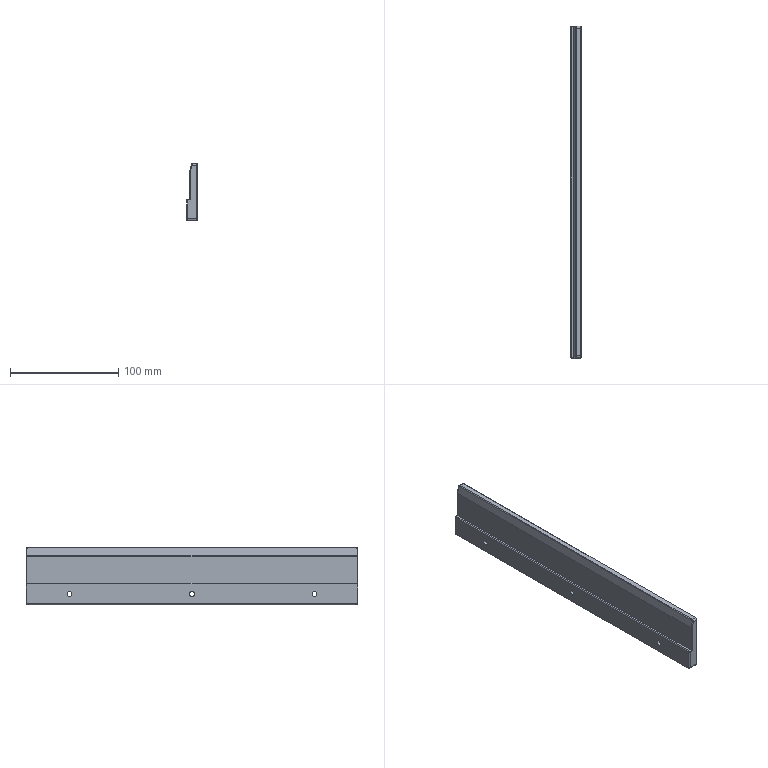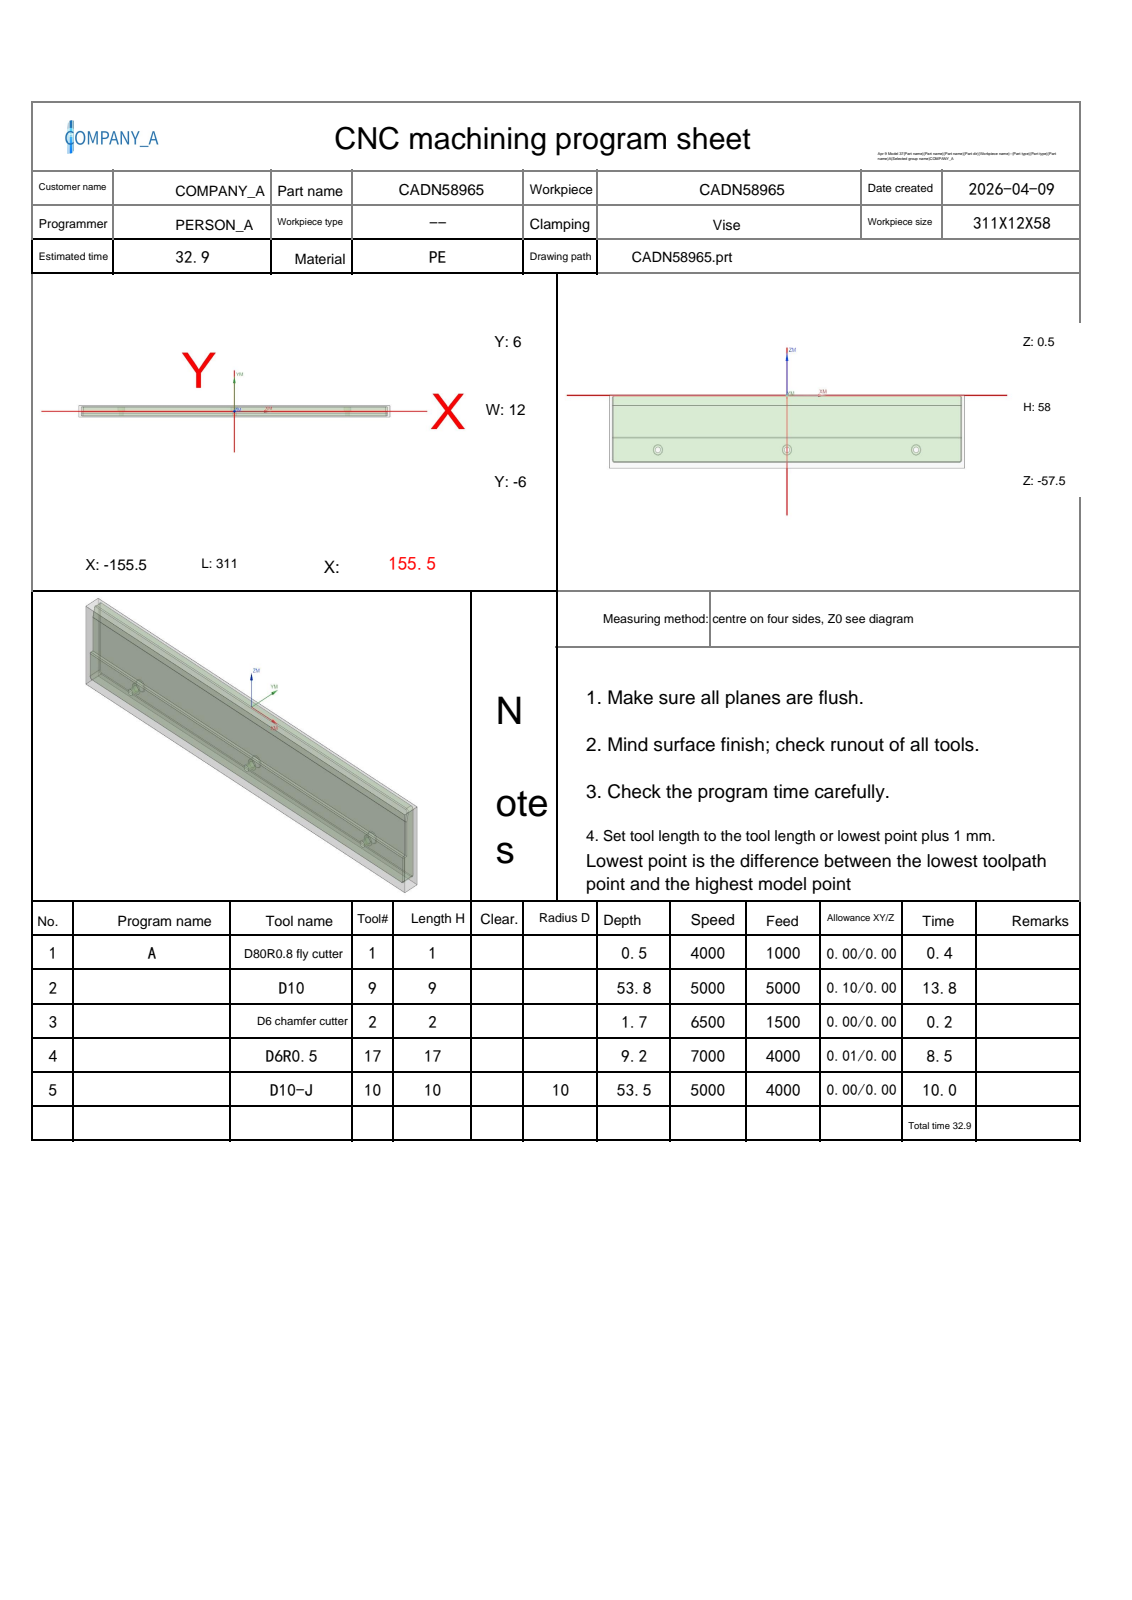NC program | NX | posted by the shop | part box 10 x 306 x 53 mm
Lines 1 to 1289 of 3792:
%
O0001
(Machine time: 34.05 MIN)
(===Total Tool:5===)
(T1=D80R0.8 fly cutter D=80.  R=0.8  D-  H01 Z=0.    )
(T9=D10     D=10.  R=0.   D-  H09 Z=-53.3 )
(T2=D6 chamfer cutter   D=6.   R=0.   D-  H02 Z=-1.2  )
(T17=D6R0.5 D=6.   R=0.5  D-  H17 Z=-8.69 )
(T10=D10-J  D=10.  R=0.   D10 H10 Z=-53.  )
G80 G90 G17 G49 G40
G91 G28 Z0
M01
N1 T01 M06
(D80R0.8 fly cutter  D=80. R=0.8 H=01 ce=0.00 di=0.00)
G00 G90 G54 X198. Y0.0 M03 S4000
G43 H01 Z20.
M08
Z2.
G01 Z0.0 F1000.
X193.
X-193.
X-198.
Z2.
G00 Z20.
G91 G28 Z0.0
M05
M09
G91 G28 Z0.0
M01
N2 T09 M06
(D10  D=10. R=0. H=09 ce=0.10 di=0.00)
G00 G90 G54 X0.0 Y10.1 M03 S5000
G43 H09 Z20.
M08
Z.5
G01 X152.5 Z.318 F5000.
G02 X156.106 Y8.606 Z.313 I0.0 J-5.1
G01 X156.606 Y8.106 Z.312
G02 X158.1 Y4.5 Z.308 I-3.606 J-3.606
G01 Y-4.25 Z.297
G02 X152.25 Y-10.1 Z.286 I-5.85 J0.0
G01 X-152.25 Z-.077
G02 X-158.1 Y-4.25 Z-.088 I0.0 J5.85
G01 Y4.5 Z-.099
G02 X-156.606 Y8.106 Z-.104 I5.1 J0.0
G01 X-156.106 Y8.606
G02 X-152.5 Y10.1 Z-.109 I3.606 J-3.606
G01 X152.5 Z-.473
G02 X156.106 Y8.606 Z-.478 I0.0 J-5.1
G01 X156.606 Y8.106 Z-.479
G02 X158.1 Y4.5 Z-.484 I-3.606 J-3.606
G01 Y-4.25 Z-.494
G02 X152.25 Y-10.1 Z-.505 I-5.85 J0.0
G01 X-152.25 Z-.869
G02 X-158.1 Y-4.25 Z-.879 I0.0 J5.85
G01 Y4.5 Z-.89
G02 X-156.606 Y8.106 Z-.895 I5.1 J0.0
G01 X-156.106 Y8.606 Z-.896
G02 X-152.5 Y10.1 Z-.9 I3.606 J-3.606
G01 X152.5 Z-1.264
G02 X156.106 Y8.606 Z-1.269 I0.0 J-5.1
G01 X156.606 Y8.106 Z-1.27
G02 X158.1 Y4.5 Z-1.275 I-3.606 J-3.606
G01 Y-4.25 Z-1.285
G02 X152.25 Y-10.1 Z-1.296 I-5.85 J0.0
G01 X-152.25 Z-1.66
G02 X-158.1 Y-4.25 Z-1.671 I0.0 J5.85
G01 Y4.5 Z-1.681
G02 X-156.606 Y8.106 Z-1.686 I5.1 J0.0
G01 X-156.106 Y8.606 Z-1.687
G02 X-152.5 Y10.1 Z-1.691 I3.606 J-3.606
G01 X152.5 Z-2.056
G02 X156.106 Y8.606 Z-2.06 I0.0 J-5.1
G01 X156.606 Y8.106 Z-2.061
G02 X158.1 Y4.5 Z-2.066 I-3.606 J-3.606
G01 Y-4.25 Z-2.076
G02 X152.25 Y-10.1 Z-2.087 I-5.85 J0.0
G01 X-152.25 Z-2.451
G02 X-158.1 Y-4.25 Z-2.462 I0.0 J5.85
G01 Y4.5 Z-2.472
G02 X-156.606 Y8.106 Z-2.477 I5.1 J0.0
G01 X-156.106 Y8.606 Z-2.478
G02 X-152.5 Y10.1 Z-2.483 I3.606 J-3.606
G01 X152.5 Z-2.847
G02 X156.106 Y8.606 Z-2.852 I0.0 J-5.1
G01 X156.606 Y8.106
G02 X158.1 Y4.5 Z-2.857 I-3.606 J-3.606
G01 Y-4.25 Z-2.868
G02 X152.25 Y-10.1 Z-2.879 I-5.85 J0.0
G01 X-152.25 Z-3.242
G02 X-158.1 Y-4.25 Z-3.253 I0.0 J5.85
G01 Y4.5 Z-3.263
G02 X-156.606 Y8.106 Z-3.268 I5.1 J0.0
G01 X-156.106 Y8.606 Z-3.269
G02 X-152.5 Y10.1 Z-3.274 I3.606 J-3.606
G01 X152.5 Z-3.638
G02 X156.106 Y8.606 Z-3.643 I0.0 J-5.1
G01 X156.606 Y8.106 Z-3.644
G02 X158.1 Y4.5 Z-3.648 I-3.606 J-3.606
G01 Y-4.25 Z-3.659
G02 X152.25 Y-10.1 Z-3.67 I-5.85 J0.0
G01 X-152.25 Z-4.033
G02 X-158.1 Y-4.25 Z-4.044 I0.0 J5.85
G01 Y4.5 Z-4.055
G02 X-156.606 Y8.106 Z-4.059 I5.1 J0.0
G01 X-156.106 Y8.606 Z-4.06
G02 X-152.5 Y10.1 Z-4.065 I3.606 J-3.606
G01 X152.5 Z-4.429
G02 X156.106 Y8.606 Z-4.434 I0.0 J-5.1
G01 X156.606 Y8.106 Z-4.435
G02 X158.1 Y4.5 Z-4.439 I-3.606 J-3.606
G01 Y-4.25 Z-4.45
G02 X152.25 Y-10.1 Z-4.461 I-5.85 J0.0
G01 X-152.25 Z-4.824
G02 X-158.1 Y-4.25 Z-4.835 I0.0 J5.85
G01 Y4.5 Z-4.846
G02 X-156.606 Y8.106 Z-4.851 I5.1 J0.0
G01 X-156.106 Y8.606
G02 X-152.5 Y10.1 Z-4.856 I3.606 J-3.606
G01 X152.5 Z-5.22
G02 X156.106 Y8.606 Z-5.225 I0.0 J-5.1
G01 X156.606 Y8.106 Z-5.226
G02 X158.1 Y4.5 Z-5.231 I-3.606 J-3.606
G01 Y-4.25 Z-5.241
G02 X152.25 Y-10.1 Z-5.252 I-5.85 J0.0
G01 X-152.25 Z-5.616
G02 X-158.1 Y-4.25 Z-5.627 I0.0 J5.85
G01 Y4.5 Z-5.637
G02 X-156.606 Y8.106 Z-5.642 I5.1 J0.0
G01 X-156.106 Y8.606 Z-5.643
G02 X-152.5 Y10.1 Z-5.647 I3.606 J-3.606
G01 X152.5 Z-6.011
G02 X156.106 Y8.606 Z-6.016 I0.0 J-5.1
G01 X156.606 Y8.106 Z-6.017
G02 X158.1 Y4.5 Z-6.022 I-3.606 J-3.606
G01 Y-4.25 Z-6.032
G02 X152.25 Y-10.1 Z-6.043 I-5.85 J0.0
G01 X-152.25 Z-6.407
G02 X-158.1 Y-4.25 Z-6.418 I0.0 J5.85
G01 Y4.5 Z-6.428
G02 X-156.606 Y8.106 Z-6.433 I5.1 J0.0
G01 X-156.106 Y8.606 Z-6.434
G02 X-152.5 Y10.1 Z-6.439 I3.606 J-3.606
G01 X152.5 Z-6.803
G02 X156.106 Y8.606 Z-6.807 I0.0 J-5.1
G01 X156.606 Y8.106 Z-6.808
G02 X158.1 Y4.5 Z-6.813 I-3.606 J-3.606
G01 Y-4.25 Z-6.823
G02 X152.25 Y-10.1 Z-6.834 I-5.85 J0.0
G01 X-152.25 Z-7.198
G02 X-158.1 Y-4.25 Z-7.209 I0.0 J5.85
G01 Y4.5 Z-7.219
G02 X-156.606 Y8.106 Z-7.224 I5.1 J0.0
G01 X-156.106 Y8.606 Z-7.225
G02 X-152.5 Y10.1 Z-7.23 I3.606 J-3.606
G01 X152.5 Z-7.594
G02 X156.106 Y8.606 Z-7.599 I0.0 J-5.1
G01 X156.606 Y8.106
G02 X158.1 Y4.5 Z-7.604 I-3.606 J-3.606
G01 Y-4.25 Z-7.615
G02 X152.25 Y-10.1 Z-7.626 I-5.85 J0.0
G01 X-152.25 Z-7.989
G02 X-158.1 Y-4.25 Z-8. I0.0 J5.85
G01 Y4.5 Z-8.011
G02 X-156.606 Y8.106 Z-8.015 I5.1 J0.0
G01 X-156.106 Y8.606 Z-8.016
G02 X-152.5 Y10.1 Z-8.021 I3.606 J-3.606
G01 X152.5 Z-8.385
G02 X156.106 Y8.606 Z-8.39 I0.0 J-5.1
G01 X156.606 Y8.106 Z-8.391
G02 X158.1 Y4.5 Z-8.395 I-3.606 J-3.606
G01 Y-4.25 Z-8.406
G02 X152.25 Y-10.1 Z-8.417 I-5.85 J0.0
G01 X-152.25 Z-8.78
G02 X-158.1 Y-4.25 Z-8.791 I0.0 J5.85
G01 Y4.5 Z-8.802
G02 X-156.606 Y8.106 Z-8.806 I5.1 J0.0
G01 X-156.106 Y8.606 Z-8.807
G02 X-152.5 Y10.1 Z-8.812 I3.606 J-3.606
G01 X152.5 Z-9.176
G02 X156.106 Y8.606 Z-9.181 I0.0 J-5.1
G01 X156.606 Y8.106 Z-9.182
G02 X158.1 Y4.5 Z-9.187 I-3.606 J-3.606
G01 Y-4.25 Z-9.197
G02 X152.25 Y-10.1 Z-9.208 I-5.85 J0.0
G01 X-152.25 Z-9.571
G02 X-158.1 Y-4.25 Z-9.582 I0.0 J5.85
G01 Y4.5 Z-9.593
G02 X-156.606 Y8.106 Z-9.598 I5.1 J0.0
G01 X-156.106 Y8.606
G02 X-152.5 Y10.1 Z-9.603 I3.606 J-3.606
G01 X152.5 Z-9.967
G02 X156.106 Y8.606 Z-9.972 I0.0 J-5.1
G01 X156.606 Y8.106 Z-9.973
G02 X158.1 Y4.5 Z-9.978 I-3.606 J-3.606
G01 Y-4.25 Z-9.988
G02 X152.25 Y-10.1 Z-9.999 I-5.85 J0.0
G01 X-152.25 Z-10.363
G02 X-158.1 Y-4.25 Z-10.374 I0.0 J5.85
G01 Y4.5 Z-10.384
G02 X-156.606 Y8.106 Z-10.389 I5.1 J0.0
G01 X-156.106 Y8.606 Z-10.39
G02 X-152.5 Y10.1 Z-10.394 I3.606 J-3.606
G01 X152.5 Z-10.759
G02 X156.106 Y8.606 Z-10.763 I0.0 J-5.1
G01 X156.606 Y8.106 Z-10.764
G02 X158.1 Y4.5 Z-10.769 I-3.606 J-3.606
G01 Y-4.25 Z-10.779
G02 X152.25 Y-10.1 Z-10.79 I-5.85 J0.0
G01 X-152.25 Z-11.154
G02 X-158.1 Y-4.25 Z-11.165 I0.0 J5.85
G01 Y4.5 Z-11.175
G02 X-156.606 Y8.106 Z-11.18 I5.1 J0.0
G01 X-156.106 Y8.606 Z-11.181
G02 X-152.5 Y10.1 Z-11.186 I3.606 J-3.606
G01 X152.5 Z-11.55
G02 X156.106 Y8.606 Z-11.554 I0.0 J-5.1
G01 X156.606 Y8.106 Z-11.555
G02 X158.1 Y4.5 Z-11.56 I-3.606 J-3.606
G01 Y-4.25 Z-11.571
G02 X152.25 Y-10.1 Z-11.582 I-5.85 J0.0
G01 X-152.25 Z-11.945
G02 X-158.1 Y-4.25 Z-11.956 I0.0 J5.85
G01 Y4.5 Z-11.966
G02 X-156.606 Y8.106 Z-11.971 I5.1 J0.0
G01 X-156.106 Y8.606 Z-11.972
G02 X-152.5 Y10.1 Z-11.977 I3.606 J-3.606
G01 X152.5 Z-12.341
G02 X156.106 Y8.606 Z-12.346 I0.0 J-5.1
G01 X156.606 Y8.106
G02 X158.1 Y4.5 Z-12.351 I-3.606 J-3.606
G01 Y-4.25 Z-12.362
G02 X152.25 Y-10.1 Z-12.373 I-5.85 J0.0
G01 X-152.25 Z-12.736
G02 X-158.1 Y-4.25 Z-12.747 I0.0 J5.85
G01 Y4.5 Z-12.758
G02 X-156.606 Y8.106 Z-12.762 I5.1 J0.0
G01 X-156.106 Y8.606 Z-12.763
G02 X-152.5 Y10.1 Z-12.768 I3.606 J-3.606
G01 X152.5 Z-13.132
G02 X156.106 Y8.606 Z-13.137 I0.0 J-5.1
G01 X156.606 Y8.106 Z-13.138
G02 X158.1 Y4.5 Z-13.142 I-3.606 J-3.606
G01 Y-4.25 Z-13.153
G02 X152.25 Y-10.1 Z-13.164 I-5.85 J0.0
G01 X-152.25 Z-13.527
G02 X-158.1 Y-4.25 Z-13.538 I0.0 J5.85
G01 Y4.5 Z-13.549
G02 X-156.606 Y8.106 Z-13.554 I5.1 J0.0
G01 X-156.106 Y8.606
G02 X-152.5 Y10.1 Z-13.559 I3.606 J-3.606
G01 X152.5 Z-13.923
G02 X156.106 Y8.606 Z-13.928 I0.0 J-5.1
G01 X156.606 Y8.106 Z-13.929
G02 X158.1 Y4.5 Z-13.934 I-3.606 J-3.606
G01 Y-4.25 Z-13.944
G02 X152.25 Y-10.1 Z-13.955 I-5.85 J0.0
G01 X-152.25 Z-14.319
G02 X-158.1 Y-4.25 Z-14.329 I0.0 J5.85
G01 Y4.5 Z-14.34
G02 X-156.606 Y8.106 Z-14.345 I5.1 J0.0
G01 X-156.106 Y8.606 Z-14.346
G02 X-152.5 Y10.1 Z-14.35 I3.606 J-3.606
G01 X152.5 Z-14.714
G02 X156.106 Y8.606 Z-14.719 I0.0 J-5.1
G01 X156.606 Y8.106 Z-14.72
G02 X158.1 Y4.5 Z-14.725 I-3.606 J-3.606
G01 Y-4.25 Z-14.735
G02 X152.25 Y-10.1 Z-14.746 I-5.85 J0.0
G01 X-152.25 Z-15.11
G02 X-158.1 Y-4.25 Z-15.121 I0.0 J5.85
G01 Y4.5 Z-15.131
G02 X-156.606 Y8.106 Z-15.136 I5.1 J0.0
G01 X-156.106 Y8.606 Z-15.137
G02 X-152.5 Y10.1 Z-15.141 I3.606 J-3.606
G01 X152.5 Z-15.506
G02 X156.106 Y8.606 Z-15.51 I0.0 J-5.1
G01 X156.606 Y8.106 Z-15.511
G02 X158.1 Y4.5 Z-15.516 I-3.606 J-3.606
G01 Y-4.25 Z-15.526
G02 X152.25 Y-10.1 Z-15.537 I-5.85 J0.0
G01 X-152.25 Z-15.901
G02 X-158.1 Y-4.25 Z-15.912 I0.0 J5.85
G01 Y4.5 Z-15.922
G02 X-156.606 Y8.106 Z-15.927 I5.1 J0.0
G01 X-156.106 Y8.606 Z-15.928
G02 X-152.5 Y10.1 Z-15.933 I3.606 J-3.606
G01 X152.5 Z-16.297
G02 X156.106 Y8.606 Z-16.302 I0.0 J-5.1
G01 X156.606 Y8.106
G02 X158.1 Y4.5 Z-16.307 I-3.606 J-3.606
G01 Y-4.25 Z-16.318
G02 X152.25 Y-10.1 Z-16.329 I-5.85 J0.0
G01 X-152.25 Z-16.692
G02 X-158.1 Y-4.25 Z-16.703 I0.0 J5.85
G01 Y4.5 Z-16.713
G02 X-156.606 Y8.106 Z-16.718 I5.1 J0.0
G01 X-156.106 Y8.606 Z-16.719
G02 X-152.5 Y10.1 Z-16.724 I3.606 J-3.606
G01 X152.5 Z-17.088
G02 X156.106 Y8.606 Z-17.093 I0.0 J-5.1
G01 X156.606 Y8.106 Z-17.094
G02 X158.1 Y4.5 Z-17.098 I-3.606 J-3.606
G01 Y-4.25 Z-17.109
G02 X152.25 Y-10.1 Z-17.12 I-5.85 J0.0
G01 X-152.25 Z-17.483
G02 X-158.1 Y-4.25 Z-17.494 I0.0 J5.85
G01 Y4.5 Z-17.505
G02 X-156.606 Y8.106 Z-17.509 I5.1 J0.0
G01 X-156.106 Y8.606 Z-17.51
G02 X-152.5 Y10.1 Z-17.515 I3.606 J-3.606
G01 X152.5 Z-17.879
G02 X156.106 Y8.606 Z-17.884 I0.0 J-5.1
G01 X156.606 Y8.106 Z-17.885
G02 X158.1 Y4.5 Z-17.889 I-3.606 J-3.606
G01 Y-4.25 Z-17.9
G02 X152.25 Y-10.1 Z-17.911 I-5.85 J0.0
G01 X-152.25 Z-18.274
G02 X-158.1 Y-4.25 Z-18.285 I0.0 J5.85
G01 Y4.5 Z-18.296
G02 X-156.606 Y8.106 Z-18.301 I5.1 J0.0
G01 X-156.106 Y8.606
G02 X-152.5 Y10.1 Z-18.306 I3.606 J-3.606
G01 X152.5 Z-18.67
G02 X156.106 Y8.606 Z-18.675 I0.0 J-5.1
G01 X156.606 Y8.106 Z-18.676
G02 X158.1 Y4.5 Z-18.681 I-3.606 J-3.606
G01 Y-4.25 Z-18.691
G02 X152.25 Y-10.1 Z-18.702 I-5.85 J0.0
G01 X-152.25 Z-19.066
G02 X-158.1 Y-4.25 Z-19.077 I0.0 J5.85
G01 Y4.5 Z-19.087
G02 X-156.606 Y8.106 Z-19.092 I5.1 J0.0
G01 X-156.106 Y8.606 Z-19.093
G02 X-152.5 Y10.1 Z-19.097 I3.606 J-3.606
G01 X152.5 Z-19.461
G02 X156.106 Y8.606 Z-19.466 I0.0 J-5.1
G01 X156.606 Y8.106 Z-19.467
G02 X158.1 Y4.5 Z-19.472 I-3.606 J-3.606
G01 Y-4.25 Z-19.482
G02 X152.25 Y-10.1 Z-19.493 I-5.85 J0.0
G01 X-152.25 Z-19.857
G02 X-158.1 Y-4.25 Z-19.868 I0.0 J5.85
G01 Y4.5 Z-19.878
G02 X-156.606 Y8.106 Z-19.883 I5.1 J0.0
G01 X-156.106 Y8.606 Z-19.884
G02 X-152.5 Y10.1 Z-19.889 I3.606 J-3.606
G01 X152.5 Z-20.253
G02 X156.106 Y8.606 Z-20.257 I0.0 J-5.1
G01 X156.606 Y8.106 Z-20.258
G02 X158.1 Y4.5 Z-20.263 I-3.606 J-3.606
G01 Y-4.25 Z-20.273
G02 X152.25 Y-10.1 Z-20.284 I-5.85 J0.0
G01 X-152.25 Z-20.648
G02 X-158.1 Y-4.25 Z-20.659 I0.0 J5.85
G01 Y4.5 Z-20.669
G02 X-156.606 Y8.106 Z-20.674 I5.1 J0.0
G01 X-156.106 Y8.606 Z-20.675
G02 X-152.5 Y10.1 Z-20.68 I3.606 J-3.606
G01 X152.5 Z-21.044
G02 X156.106 Y8.606 Z-21.049 I0.0 J-5.1
G01 X156.606 Y8.106
G02 X158.1 Y4.5 Z-21.054 I-3.606 J-3.606
G01 Y-4.25 Z-21.065
G02 X152.25 Y-10.1 Z-21.076 I-5.85 J0.0
G01 X-152.25 Z-21.439
G02 X-158.1 Y-4.25 Z-21.45 I0.0 J5.85
G01 Y4.5 Z-21.461
G02 X-156.606 Y8.106 Z-21.465 I5.1 J0.0
G01 X-156.106 Y8.606 Z-21.466
G02 X-152.5 Y10.1 Z-21.471 I3.606 J-3.606
G01 X152.5 Z-21.835
G02 X156.106 Y8.606 Z-21.84 I0.0 J-5.1
G01 X156.606 Y8.106 Z-21.841
G02 X158.1 Y4.5 Z-21.845 I-3.606 J-3.606
G01 Y-4.25 Z-21.856
G02 X152.25 Y-10.1 Z-21.867 I-5.85 J0.0
G01 X-152.25 Z-22.23
G02 X-158.1 Y-4.25 Z-22.241 I0.0 J5.85
G01 Y4.5 Z-22.252
G02 X-156.606 Y8.106 Z-22.256 I5.1 J0.0
G01 X-156.106 Y8.606 Z-22.257
G02 X-152.5 Y10.1 Z-22.262 I3.606 J-3.606
G01 X152.5 Z-22.626
G02 X156.106 Y8.606 Z-22.631 I0.0 J-5.1
G01 X156.606 Y8.106 Z-22.632
G02 X158.1 Y4.5 Z-22.637 I-3.606 J-3.606
G01 Y-4.25 Z-22.647
G02 X152.25 Y-10.1 Z-22.658 I-5.85 J0.0
G01 X-152.25 Z-23.021
G02 X-158.1 Y-4.25 Z-23.032 I0.0 J5.85
G01 Y4.5 Z-23.043
G02 X-156.606 Y8.106 Z-23.048 I5.1 J0.0
G01 X-156.106 Y8.606
G02 X-152.5 Y10.1 Z-23.053 I3.606 J-3.606
G01 X152.5 Z-23.417
G02 X156.106 Y8.606 Z-23.422 I0.0 J-5.1
G01 X156.606 Y8.106 Z-23.423
G02 X158.1 Y4.5 Z-23.428 I-3.606 J-3.606
G01 Y-4.25 Z-23.438
G02 X152.25 Y-10.1 Z-23.449 I-5.85 J0.0
G01 X-152.25 Z-23.813
G02 X-158.1 Y-4.25 Z-23.824 I0.0 J5.85
G01 Y4.5 Z-23.834
G02 X-156.606 Y8.106 Z-23.839 I5.1 J0.0
G01 X-156.106 Y8.606 Z-23.84
G02 X-152.5 Y10.1 Z-23.844 I3.606 J-3.606
G01 X152.5 Z-24.209
G02 X156.106 Y8.606 Z-24.213 I0.0 J-5.1
G01 X156.606 Y8.106 Z-24.214
G02 X158.1 Y4.5 Z-24.219 I-3.606 J-3.606
G01 Y-4.25 Z-24.229
G02 X152.25 Y-10.1 Z-24.24 I-5.85 J0.0
G01 X-152.25 Z-24.604
G02 X-158.1 Y-4.25 Z-24.615 I0.0 J5.85
G01 Y4.5 Z-24.625
G02 X-156.606 Y8.106 Z-24.63 I5.1 J0.0
G01 X-156.106 Y8.606 Z-24.631
G02 X-152.5 Y10.1 Z-24.636 I3.606 J-3.606
G01 X152.5 Z-25.
G02 X156.106 Y8.606 Z-25.004 I0.0 J-5.1
G01 X156.606 Y8.106 Z-25.005
G02 X158.1 Y4.5 Z-25.01 I-3.606 J-3.606
G01 Y-4.25 Z-25.021
G02 X152.25 Y-10.1 Z-25.032 I-5.85 J0.0
G01 X-152.25 Z-25.395
G02 X-158.1 Y-4.25 Z-25.406 I0.0 J5.85
G01 Y4.5 Z-25.416
G02 X-156.606 Y8.106 Z-25.421 I5.1 J0.0
G01 X-156.106 Y8.606 Z-25.422
G02 X-152.5 Y10.1 Z-25.427 I3.606 J-3.606
G01 X152.5 Z-25.791
G02 X156.106 Y8.606 Z-25.796 I0.0 J-5.1
G01 X156.606 Y8.106
G02 X158.1 Y4.5 Z-25.801 I-3.606 J-3.606
G01 Y-4.25 Z-25.812
G02 X152.25 Y-10.1 Z-25.823 I-5.85 J0.0
G01 X-152.25 Z-26.186
G02 X-158.1 Y-4.25 Z-26.197 I0.0 J5.85
G01 Y4.5 Z-26.208
G02 X-156.606 Y8.106 Z-26.212 I5.1 J0.0
G01 X-156.106 Y8.606 Z-26.213
G02 X-152.5 Y10.1 Z-26.218 I3.606 J-3.606
G01 X152.5 Z-26.582
G02 X156.106 Y8.606 Z-26.587 I0.0 J-5.1
G01 X156.606 Y8.106 Z-26.588
G02 X158.1 Y4.5 Z-26.592 I-3.606 J-3.606
G01 Y-4.25 Z-26.603
G02 X152.25 Y-10.1 Z-26.614 I-5.85 J0.0
G01 X-152.25 Z-26.977
G02 X-158.1 Y-4.25 Z-26.988 I0.0 J5.85
G01 Y4.5 Z-26.999
G02 X-156.606 Y8.106 Z-27.004 I5.1 J0.0
G01 X-156.106 Y8.606
G02 X-152.5 Y10.1 Z-27.009 I3.606 J-3.606
G01 X152.5 Z-27.373
G02 X156.106 Y8.606 Z-27.378 I0.0 J-5.1
G01 X156.606 Y8.106 Z-27.379
G02 X158.1 Y4.5 Z-27.384 I-3.606 J-3.606
G01 Y-4.25 Z-27.394
G02 X152.25 Y-10.1 Z-27.405 I-5.85 J0.0
G01 X-152.25 Z-27.769
G02 X-158.1 Y-4.25 Z-27.779 I0.0 J5.85
G01 Y4.5 Z-27.79
G02 X-156.606 Y8.106 Z-27.795 I5.1 J0.0
G01 X-156.106 Y8.606 Z-27.796
G02 X-152.5 Y10.1 Z-27.8 I3.606 J-3.606
G01 X152.5 Z-28.164
G02 X156.106 Y8.606 Z-28.169 I0.0 J-5.1
G01 X156.606 Y8.106 Z-28.17
G02 X158.1 Y4.5 Z-28.175 I-3.606 J-3.606
G01 Y-4.25 Z-28.185
G02 X152.25 Y-10.1 Z-28.196 I-5.85 J0.0
G01 X-152.25 Z-28.56
G02 X-158.1 Y-4.25 Z-28.571 I0.0 J5.85
G01 Y4.5 Z-28.581
G02 X-156.606 Y8.106 Z-28.586 I5.1 J0.0
G01 X-156.106 Y8.606 Z-28.587
G02 X-152.5 Y10.1 Z-28.591 I3.606 J-3.606
G01 X152.5 Z-28.956
G02 X156.106 Y8.606 Z-28.96 I0.0 J-5.1
G01 X156.606 Y8.106 Z-28.961
G02 X158.1 Y4.5 Z-28.966 I-3.606 J-3.606
G01 Y-4.25 Z-28.976
G02 X152.25 Y-10.1 Z-28.987 I-5.85 J0.0
G01 X-152.25 Z-29.351
G02 X-158.1 Y-4.25 Z-29.362 I0.0 J5.85
G01 Y4.5 Z-29.372
G02 X-156.606 Y8.106 Z-29.377 I5.1 J0.0
G01 X-156.106 Y8.606 Z-29.378
G02 X-152.5 Y10.1 Z-29.383 I3.606 J-3.606
G01 X152.5 Z-29.747
G02 X156.106 Y8.606 Z-29.752 I0.0 J-5.1
G01 X156.606 Y8.106
G02 X158.1 Y4.5 Z-29.757 I-3.606 J-3.606
G01 Y-4.25 Z-29.768
G02 X152.25 Y-10.1 Z-29.779 I-5.85 J0.0
G01 X-152.25 Z-30.142
G02 X-158.1 Y-4.25 Z-30.153 I0.0 J5.85
G01 Y4.5 Z-30.163
G02 X-156.606 Y8.106 Z-30.168 I5.1 J0.0
G01 X-156.106 Y8.606 Z-30.169
G02 X-152.5 Y10.1 Z-30.174 I3.606 J-3.606
G01 X152.5 Z-30.538
G02 X156.106 Y8.606 Z-30.543 I0.0 J-5.1
G01 X156.606 Y8.106 Z-30.544
G02 X158.1 Y4.5 Z-30.548 I-3.606 J-3.606
G01 Y-4.25 Z-30.559
G02 X152.25 Y-10.1 Z-30.57 I-5.85 J0.0
G01 X-152.25 Z-30.933
G02 X-158.1 Y-4.25 Z-30.944 I0.0 J5.85
G01 Y4.5 Z-30.955
G02 X-156.606 Y8.106 Z-30.959 I5.1 J0.0
G01 X-156.106 Y8.606 Z-30.96
G02 X-152.5 Y10.1 Z-30.965 I3.606 J-3.606
G01 X152.5 Z-31.329
G02 X156.106 Y8.606 Z-31.334 I0.0 J-5.1
G01 X156.606 Y8.106 Z-31.335
G02 X158.1 Y4.5 Z-31.339 I-3.606 J-3.606
G01 Y-4.25 Z-31.35
G02 X152.25 Y-10.1 Z-31.361 I-5.85 J0.0
G01 X-152.25 Z-31.724
G02 X-158.1 Y-4.25 Z-31.735 I0.0 J5.85
G01 Y4.5 Z-31.746
G02 X-156.606 Y8.106 Z-31.751 I5.1 J0.0
G01 X-156.106 Y8.606
G02 X-152.5 Y10.1 Z-31.756 I3.606 J-3.606
G01 X152.5 Z-32.12
G02 X156.106 Y8.606 Z-32.125 I0.0 J-5.1
G01 X156.606 Y8.106 Z-32.126
G02 X158.1 Y4.5 Z-32.131 I-3.606 J-3.606
G01 Y-4.25 Z-32.141
G02 X152.25 Y-10.1 Z-32.152 I-5.85 J0.0
G01 X-152.25 Z-32.516
G02 X-158.1 Y-4.25 Z-32.527 I0.0 J5.85
G01 Y4.5 Z-32.537
G02 X-156.606 Y8.106 Z-32.542 I5.1 J0.0
G01 X-156.106 Y8.606 Z-32.543
G02 X-152.5 Y10.1 Z-32.547 I3.606 J-3.606
G01 X152.5 Z-32.911
G02 X156.106 Y8.606 Z-32.916 I0.0 J-5.1
G01 X156.606 Y8.106 Z-32.917
G02 X158.1 Y4.5 Z-32.922 I-3.606 J-3.606
G01 Y-4.25 Z-32.932
G02 X152.25 Y-10.1 Z-32.943 I-5.85 J0.0
G01 X-152.25 Z-33.307
G02 X-158.1 Y-4.25 Z-33.318 I0.0 J5.85
G01 Y4.5 Z-33.328
G02 X-156.606 Y8.106 Z-33.333 I5.1 J0.0
G01 X-156.106 Y8.606 Z-33.334
G02 X-152.5 Y10.1 Z-33.339 I3.606 J-3.606
G01 X152.5 Z-33.703
G02 X156.106 Y8.606 Z-33.707 I0.0 J-5.1
G01 X156.606 Y8.106 Z-33.708
G02 X158.1 Y4.5 Z-33.713 I-3.606 J-3.606
G01 Y-4.25 Z-33.723
G02 X152.25 Y-10.1 Z-33.734 I-5.85 J0.0
G01 X-152.25 Z-34.098
G02 X-158.1 Y-4.25 Z-34.109 I0.0 J5.85
G01 Y4.5 Z-34.119
G02 X-156.606 Y8.106 Z-34.124 I5.1 J0.0
G01 X-156.106 Y8.606 Z-34.125
G02 X-152.5 Y10.1 Z-34.13 I3.606 J-3.606
G01 X152.5 Z-34.494
G02 X156.106 Y8.606 Z-34.499 I0.0 J-5.1
G01 X156.606 Y8.106
G02 X158.1 Y4.5 Z-34.504 I-3.606 J-3.606
G01 Y-4.25 Z-34.515
G02 X152.25 Y-10.1 Z-34.526 I-5.85 J0.0
G01 X-152.25 Z-34.889
G02 X-158.1 Y-4.25 Z-34.9 I0.0 J5.85
G01 Y4.5 Z-34.911
G02 X-156.606 Y8.106 Z-34.915 I5.1 J0.0
G01 X-156.106 Y8.606 Z-34.916
G02 X-152.5 Y10.1 Z-34.921 I3.606 J-3.606
G01 X152.5 Z-35.285
G02 X156.106 Y8.606 Z-35.29 I0.0 J-5.1
G01 X156.606 Y8.106 Z-35.291
G02 X158.1 Y4.5 Z-35.295 I-3.606 J-3.606
G01 Y-4.25 Z-35.306
G02 X152.25 Y-10.1 Z-35.317 I-5.85 J0.0
G01 X-152.25 Z-35.68
G02 X-158.1 Y-4.25 Z-35.691 I0.0 J5.85
G01 Y4.5 Z-35.702
G02 X-156.606 Y8.106 Z-35.706 I5.1 J0.0
G01 X-156.106 Y8.606 Z-35.707
G02 X-152.5 Y10.1 Z-35.712 I3.606 J-3.606
G01 X152.5 Z-36.076
G02 X156.106 Y8.606 Z-36.081 I0.0 J-5.1
G01 X156.606 Y8.106 Z-36.082
G02 X158.1 Y4.5 Z-36.087 I-3.606 J-3.606
G01 Y-4.25 Z-36.097
G02 X152.25 Y-10.1 Z-36.108 I-5.85 J0.0
G01 X-152.25 Z-36.471
G02 X-158.1 Y-4.25 Z-36.482 I0.0 J5.85
G01 Y4.5 Z-36.493
G02 X-156.606 Y8.106 Z-36.498 I5.1 J0.0
G01 X-156.106 Y8.606
G02 X-152.5 Y10.1 Z-36.503 I3.606 J-3.606
G01 X152.5 Z-36.867
G02 X156.106 Y8.606 Z-36.872 I0.0 J-5.1
G01 X156.606 Y8.106 Z-36.873
G02 X158.1 Y4.5 Z-36.878 I-3.606 J-3.606
G01 Y-4.25 Z-36.888
G02 X152.25 Y-10.1 Z-36.899 I-5.85 J0.0
G01 X-152.25 Z-37.263
G02 X-158.1 Y-4.25 Z-37.274 I0.0 J5.85
G01 Y4.5 Z-37.284
G02 X-156.606 Y8.106 Z-37.289 I5.1 J0.0
G01 X-156.106 Y8.606 Z-37.29
G02 X-152.5 Y10.1 Z-37.294 I3.606 J-3.606
G01 X152.5 Z-37.659
G02 X156.106 Y8.606 Z-37.663 I0.0 J-5.1
G01 X156.606 Y8.106 Z-37.664
G02 X158.1 Y4.5 Z-37.669 I-3.606 J-3.606
G01 Y-4.25 Z-37.679
G02 X152.25 Y-10.1 Z-37.69 I-5.85 J0.0
G01 X-152.25 Z-38.054
G02 X-158.1 Y-4.25 Z-38.065 I0.0 J5.85
G01 Y4.5 Z-38.075
G02 X-156.606 Y8.106 Z-38.08 I5.1 J0.0
G01 X-156.106 Y8.606 Z-38.081
G02 X-152.5 Y10.1 Z-38.086 I3.606 J-3.606
G01 X152.5 Z-38.45
G02 X156.106 Y8.606 Z-38.454 I0.0 J-5.1
G01 X156.606 Y8.106 Z-38.455
G02 X158.1 Y4.5 Z-38.46 I-3.606 J-3.606
G01 Y-4.25 Z-38.471
G02 X152.25 Y-10.1 Z-38.482 I-5.85 J0.0
G01 X-152.25 Z-38.845
G02 X-158.1 Y-4.25 Z-38.856 I0.0 J5.85
G01 Y4.5 Z-38.866
G02 X-156.606 Y8.106 Z-38.871 I5.1 J0.0
G01 X-156.106 Y8.606 Z-38.872
G02 X-152.5 Y10.1 Z-38.877 I3.606 J-3.606
G01 X152.5 Z-39.241
G02 X156.106 Y8.606 Z-39.246 I0.0 J-5.1
G01 X156.606 Y8.106
G02 X158.1 Y4.5 Z-39.251 I-3.606 J-3.606
G01 Y-4.25 Z-39.262
G02 X152.25 Y-10.1 Z-39.273 I-5.85 J0.0
G01 X-152.25 Z-39.636
G02 X-158.1 Y-4.25 Z-39.647 I0.0 J5.85
G01 Y4.5 Z-39.658
G02 X-156.606 Y8.106 Z-39.662 I5.1 J0.0
G01 X-156.106 Y8.606 Z-39.663
G02 X-152.5 Y10.1 Z-39.668 I3.606 J-3.606
G01 X152.5 Z-40.032
G02 X156.106 Y8.606 Z-40.037 I0.0 J-5.1
G01 X156.606 Y8.106 Z-40.038
G02 X158.1 Y4.5 Z-40.042 I-3.606 J-3.606
G01 Y-4.25 Z-40.053
G02 X152.25 Y-10.1 Z-40.064 I-5.85 J0.0
G01 X-152.25 Z-40.427
G02 X-158.1 Y-4.25 Z-40.438 I0.0 J5.85
G01 Y4.5 Z-40.449
G02 X-156.606 Y8.106 Z-40.454 I5.1 J0.0
G01 X-156.106 Y8.606
G02 X-152.5 Y10.1 Z-40.459 I3.606 J-3.606
G01 X152.5 Z-40.823
G02 X156.106 Y8.606 Z-40.828 I0.0 J-5.1
G01 X156.606 Y8.106 Z-40.829
G02 X158.1 Y4.5 Z-40.834 I-3.606 J-3.606
G01 Y-4.25 Z-40.844
G02 X152.25 Y-10.1 Z-40.855 I-5.85 J0.0
G01 X-152.25 Z-41.219
G02 X-158.1 Y-4.25 Z-41.229 I0.0 J5.85
G01 Y4.5 Z-41.24
G02 X-156.606 Y8.106 Z-41.245 I5.1 J0.0
G01 X-156.106 Y8.606 Z-41.246
G02 X-152.5 Y10.1 Z-41.25 I3.606 J-3.606
G01 X152.5 Z-41.614
G02 X156.106 Y8.606 Z-41.619 I0.0 J-5.1
G01 X156.606 Y8.106 Z-41.62
G02 X158.1 Y4.5 Z-41.625 I-3.606 J-3.606
G01 Y-4.25 Z-41.635
G02 X152.25 Y-10.1 Z-41.646 I-5.85 J0.0
G01 X-152.25 Z-42.01
G02 X-158.1 Y-4.25 Z-42.021 I0.0 J5.85
G01 Y4.5 Z-42.031
G02 X-156.606 Y8.106 Z-42.036 I5.1 J0.0
G01 X-156.106 Y8.606 Z-42.037
G02 X-152.5 Y10.1 Z-42.041 I3.606 J-3.606
G01 X152.5 Z-42.406
G02 X156.106 Y8.606 Z-42.41 I0.0 J-5.1
G01 X156.606 Y8.106 Z-42.411
G02 X158.1 Y4.5 Z-42.416 I-3.606 J-3.606
G01 Y-4.25 Z-42.426
G02 X152.25 Y-10.1 Z-42.437 I-5.85 J0.0
G01 X-152.25 Z-42.801
G02 X-158.1 Y-4.25 Z-42.812 I0.0 J5.85
G01 Y4.5 Z-42.822
G02 X-156.606 Y8.106 Z-42.827 I5.1 J0.0
G01 X-156.106 Y8.606 Z-42.828
G02 X-152.5 Y10.1 Z-42.833 I3.606 J-3.606
G01 X152.5 Z-43.197
G02 X156.106 Y8.606 Z-43.202 I0.0 J-5.1
G01 X156.606 Y8.106
G02 X158.1 Y4.5 Z-43.207 I-3.606 J-3.606
G01 Y-4.25 Z-43.218
G02 X152.25 Y-10.1 Z-43.229 I-5.85 J0.0
G01 X-152.25 Z-43.592
G02 X-158.1 Y-4.25 Z-43.603 I0.0 J5.85
G01 Y4.5 Z-43.613
G02 X-156.606 Y8.106 Z-43.618 I5.1 J0.0
G01 X-156.106 Y8.606 Z-43.619
G02 X-152.5 Y10.1 Z-43.624 I3.606 J-3.606
G01 X152.5 Z-43.988
G02 X156.106 Y8.606 Z-43.993 I0.0 J-5.1
G01 X156.606 Y8.106 Z-43.994
G02 X158.1 Y4.5 Z-43.998 I-3.606 J-3.606
G01 Y-4.25 Z-44.009
G02 X152.25 Y-10.1 Z-44.02 I-5.85 J0.0
G01 X-152.25 Z-44.383
G02 X-158.1 Y-4.25 Z-44.394 I0.0 J5.85
G01 Y4.5 Z-44.405
G02 X-156.606 Y8.106 Z-44.409 I5.1 J0.0
G01 X-156.106 Y8.606 Z-44.41
G02 X-152.5 Y10.1 Z-44.415 I3.606 J-3.606
G01 X152.5 Z-44.779
G02 X156.106 Y8.606 Z-44.784 I0.0 J-5.1
G01 X156.606 Y8.106 Z-44.785
G02 X158.1 Y4.5 Z-44.789 I-3.606 J-3.606
G01 Y-4.25 Z-44.8
G02 X152.25 Y-10.1 Z-44.811 I-5.85 J0.0
G01 X-152.25 Z-45.174
G02 X-158.1 Y-4.25 Z-45.185 I0.0 J5.85
G01 Y4.5 Z-45.196
G02 X-156.606 Y8.106 Z-45.201 I5.1 J0.0
G01 X-156.106 Y8.606
G02 X-152.5 Y10.1 Z-45.206 I3.606 J-3.606
G01 X152.5 Z-45.57
G02 X156.106 Y8.606 Z-45.575 I0.0 J-5.1
G01 X156.606 Y8.106 Z-45.576
G02 X158.1 Y4.5 Z-45.581 I-3.606 J-3.606
G01 Y-4.25 Z-45.591
G02 X152.25 Y-10.1 Z-45.602 I-5.85 J0.0
G01 X-152.25 Z-45.966
G02 X-158.1 Y-4.25 Z-45.977 I0.0 J5.85
G01 Y4.5 Z-45.987
G02 X-156.606 Y8.106 Z-45.992 I5.1 J0.0
G01 X-156.106 Y8.606 Z-45.993
G02 X-152.5 Y10.1 Z-45.997 I3.606 J-3.606
G01 X152.5 Z-46.361
G02 X156.106 Y8.606 Z-46.366 I0.0 J-5.1
G01 X156.606 Y8.106 Z-46.367
G02 X158.1 Y4.5 Z-46.372 I-3.606 J-3.606
G01 Y-4.25 Z-46.382
G02 X152.25 Y-10.1 Z-46.393 I-5.85 J0.0
G01 X-152.25 Z-46.757
G02 X-158.1 Y-4.25 Z-46.768 I0.0 J5.85
G01 Y4.5 Z-46.778
G02 X-156.606 Y8.106 Z-46.783 I5.1 J0.0
G01 X-156.106 Y8.606 Z-46.784
G02 X-152.5 Y10.1 Z-46.789 I3.606 J-3.606
G01 X152.5 Z-47.153
G02 X156.106 Y8.606 Z-47.157 I0.0 J-5.1
G01 X156.606 Y8.106 Z-47.158
G02 X158.1 Y4.5 Z-47.163 I-3.606 J-3.606
G01 Y-4.25 Z-47.173
G02 X152.25 Y-10.1 Z-47.184 I-5.85 J0.0
G01 X-152.25 Z-47.548
G02 X-158.1 Y-4.25 Z-47.559 I0.0 J5.85
G01 Y4.5 Z-47.569
G02 X-156.606 Y8.106 Z-47.574 I5.1 J0.0
G01 X-156.106 Y8.606 Z-47.575
G02 X-152.5 Y10.1 Z-47.58 I3.606 J-3.606
G01 X152.5 Z-47.944
G02 X156.106 Y8.606 Z-47.949 I0.0 J-5.1
G01 X156.606 Y8.106
G02 X158.1 Y4.5 Z-47.954 I-3.606 J-3.606
G01 Y-4.25 Z-47.965
G02 X152.25 Y-10.1 Z-47.976 I-5.85 J0.0
G01 X-152.25 Z-48.339
G02 X-158.1 Y-4.25 Z-48.35 I0.0 J5.85
G01 Y4.5 Z-48.361
G02 X-156.606 Y8.106 Z-48.365 I5.1 J0.0
G01 X-156.106 Y8.606 Z-48.366
G02 X-152.5 Y10.1 Z-48.371 I3.606 J-3.606
G01 X152.5 Z-48.735
G02 X156.106 Y8.606 Z-48.74 I0.0 J-5.1
G01 X156.606 Y8.106 Z-48.741
G02 X158.1 Y4.5 Z-48.745 I-3.606 J-3.606
G01 Y-4.25 Z-48.756
G02 X152.25 Y-10.1 Z-48.767 I-5.85 J0.0
G01 X-152.25 Z-49.13
G02 X-158.1 Y-4.25 Z-49.141 I0.0 J5.85
G01 Y4.5 Z-49.152
G02 X-156.606 Y8.106 Z-49.156 I5.1 J0.0
G01 X-156.106 Y8.606 Z-49.157
G02 X-152.5 Y10.1 Z-49.162 I3.606 J-3.606
G01 X152.5 Z-49.526
G02 X156.106 Y8.606 Z-49.531 I0.0 J-5.1
G01 X156.606 Y8.106 Z-49.532
G02 X158.1 Y4.5 Z-49.537 I-3.606 J-3.606
G01 Y-4.25 Z-49.547
G02 X152.25 Y-10.1 Z-49.558 I-5.85 J0.0
G01 X-152.25 Z-49.921
G02 X-158.1 Y-4.25 Z-49.932 I0.0 J5.85
G01 Y4.5 Z-49.943
G02 X-156.606 Y8.106 Z-49.948 I5.1 J0.0
G01 X-156.106 Y8.606
G02 X-152.5 Y10.1 Z-49.953 I3.606 J-3.606
G01 X152.5 Z-50.317
G02 X156.106 Y8.606 Z-50.322 I0.0 J-5.1
G01 X156.606 Y8.106 Z-50.323
G02 X158.1 Y4.5 Z-50.328 I-3.606 J-3.606
G01 Y-4.25 Z-50.338
G02 X152.25 Y-10.1 Z-50.349 I-5.85 J0.0
G01 X-152.25 Z-50.713
G02 X-158.1 Y-4.25 Z-50.724 I0.0 J5.85
G01 Y4.5 Z-50.734
G02 X-156.606 Y8.106 Z-50.739 I5.1 J0.0
G01 X-156.106 Y8.606 Z-50.74
G02 X-152.5 Y10.1 Z-50.744 I3.606 J-3.606
G01 X152.5 Z-51.109
G02 X156.106 Y8.606 Z-51.113 I0.0 J-5.1
G01 X156.606 Y8.106 Z-51.114
G02 X158.1 Y4.5 Z-51.119 I-3.606 J-3.606
G01 Y-4.25 Z-51.129
G02 X152.25 Y-10.1 Z-51.14 I-5.85 J0.0
G01 X-152.25 Z-51.504
G02 X-158.1 Y-4.25 Z-51.515 I0.0 J5.85
G01 Y4.5 Z-51.525
G02 X-156.606 Y8.106 Z-51.53 I5.1 J0.0
G01 X-156.106 Y8.606 Z-51.531
G02 X-152.5 Y10.1 Z-51.536 I3.606 J-3.606
G01 X152.5 Z-51.9
G02 X156.106 Y8.606 Z-51.904 I0.0 J-5.1
G01 X156.606 Y8.106 Z-51.905
G02 X158.1 Y4.5 Z-51.91 I-3.606 J-3.606
G01 Y-4.25 Z-51.921
G02 X152.25 Y-10.1 Z-51.932 I-5.85 J0.0
G01 X-152.25 Z-52.295
G02 X-158.1 Y-4.25 Z-52.306 I0.0 J5.85
G01 Y4.5 Z-52.316
G02 X-156.606 Y8.106 Z-52.321 I5.1 J0.0
G01 X-156.106 Y8.606 Z-52.322
G02 X-152.5 Y10.1 Z-52.327 I3.606 J-3.606
G01 X152.5 Z-52.691
G02 X156.106 Y8.606 Z-52.696 I0.0 J-5.1
G01 X156.606 Y8.106
G02 X158.1 Y4.5 Z-52.701 I-3.606 J-3.606
G01 Y-4.25 Z-52.712
G02 X152.25 Y-10.1 Z-52.723 I-5.85 J0.0
G01 X-152.25 Z-53.086
G02 X-158.1 Y-4.25 Z-53.097 I0.0 J5.85
G01 Y4.5 Z-53.108
G02 X-156.606 Y8.106 Z-53.112 I5.1 J0.0
G01 X-156.106 Y8.606 Z-53.113
G02 X-152.5 Y10.1 Z-53.118 I3.606 J-3.606
G01 X0.0 Z-53.3
X152.5
G02 X156.106 Y8.606 I0.0 J-5.1
G01 X156.606 Y8.106
G02 X158.1 Y4.5 I-3.606 J-3.606
G01 Y-4.25
G02 X152.25 Y-10.1 I-5.85 J0.0
G01 X-152.25
G02 X-158.1 Y-4.25 I0.0 J5.85
G01 Y4.5
G02 X-156.606 Y8.106 I5.1 J0.0
G01 X-156.106 Y8.606
G02 X-152.5 Y10.1 I3.606 J-3.606
G01 X0.0
X.5
Z-52.3
G00 Z20.
G00 G90 X162.533 Y5.252 M03 S5000
Z20.
Z-.6
G03 X157.565 Y.26 I.032 J-5. F4000.
G02 X152.28 Y-5.478 I-5.766 J.009
G01 X151.38 Y-5.553
X-151.38
X-151.498 Y-5.554
G02 X-155.01 Y-4.534 I0.0 J6.56
X-157.565 Y.26 I3.28 J4.826
G03 X-162.535 Y5.232 I-5. J-.027
G00 X-162.928 Y4.982
Z-1.2
G02 X-157.942 Y.091 I-.012 J-5.
G03 X-157.802 Y-1.1 I6.31 J.138
X-152.102 Y-5.703 I5.7 J1.227
G01 X152.102
G03 X157.942 Y.091 I-.005 J5.845
G02 X162.924 Y5.047 I5. J-.044
G00 X163.074 Y4.992
Z-1.8
G03 X158.09 Y.003 I.016 J-5.
G02 X153.343 Y-5.729 I-5.848 J.012
X152.25 Y-5.853 I-1.361 J7.103
G01 X-152.25
G02 X-156.376 Y-4.133 I.068 J5.971
X-158.09 Y.003 I4.27 J4.193
G03 X-163.076 Y4.954 I-5. J-.049
G00 X-163.093 Y4.874
Z-2.4
G02 X-158.1 Y-.126 I-.007 J-5.
G01 Y-.127
Y-.128
G03 X-152.25 Y-6.003 I5.875 J0.0
G01 X152.25
G03 X158.1 Y-.129 I-.024 J5.874
G01 Y-.127
Y-.125
G02 X163.093 Y4.875 I5. J0.0
G00 X163.098 Y4.707
Z-3.
G03 X158.1 Y-.277 I.002 J-5.
G02 X152.205 Y-6.153 I-5.895 J.019
G01 X152.185
X-152.185
X-152.205
G02 X-158.1 Y-.277 I0.0 J5.896
G03 X-163.098 Y4.707 I-5. J-.016
G00 X-163.1 Y4.346
Z-3.6
G01 X-163.095
G02 X-158.1 Y-.427 I0.0 J-5.
G01 X-158.086 Y-.727
G03 X-152.25 Y-6.303 I5.856 J.286
G01 X152.25
G03 X156.057 Y-4.884 I-.037 J5.915
X158.1 Y-.427 I-3.946 J4.506
G02 X163.1 Y4.533 I5. J-.04
G00 Y4.353
Z-4.2
G03 X158.1 Y-.577 I0.0 J-5.
G02 X156.557 Y-4.554 I-6.114 J.085
X152.25 Y-6.453 I-4.338 J4.003
G01 X-152.25
G02 X-158.012 Y-1.549 I.017 J5.858
G01 X-158.097 Y-.68
X-158.1 Y-.577
G03 X-163.098 Y4.279 I-4.998 J-.145
G01 X-163.1
G00 Y4.009
Z-4.8
G01 X-163.093
G02 X-158.1 Y-.727 I0.0 J-5.
G01 X-158.089 Y-.927
X-157.985 Y-1.878
G03 X-152.25 Y-6.603 I5.762 J1.151
G01 X152.25
G03 X156.17 Y-5.087 I-.036 J5.918
X158.1 Y-.727 I-4.131 J4.436
G02 X163.1 Y4.21 I5. J-.063
G00 Y4.072
Z-5.4
G03 X158.1 Y-.877 I0.0 J-5.
G02 X156.17 Y-5.237 I-6.027 J.061
X152.25 Y-6.753 I-3.957 J4.404
G01 X-152.25
G02 X-158.1 Y-.877 I.045 J5.895
G03 X-163.1 Y4.107 I-5. J-.016
G00 Y3.806
Z-6.
G01 X-163.097
G02 X-158.1 Y-1.027 I0.0 J-5.
G03 X-157.858 Y-2.626 I6.926 J.231
X-152.252 Y-6.903 I5.606 J1.534
G01 X152.25
G03 X156.299 Y-5.268 I-.036 J5.92
X158.1 Y-1.027 I-4.296 J4.328
G02 X163.099 Y3.902 I4.999 J-.071
G00 X163.1 Y3.765
Z-6.6
G03 X158.1 Y-1.177 I0.0 J-5.
G02 X156.17 Y-5.537 I-6.048 J.07
X152.25 Y-7.053 I-3.96 J4.412
G01 X-152.25
G02 X-158.069 Y-1.55 I.016 J5.846
G01 X-158.1 Y-1.177
G03 X-163.083 Y3.413 I-4.983 J-.411
G01 X-163.1
G00 Y3.667
Z-7.2
G02 X-158.1 Y-1.327 I0.0 J-5.
G03 X-152.25 Y-7.203 I5.883 J.007
G01 X152.25
G03 X158.1 Y-1.327 I-.035 J5.885
G02 X163.1 Y3.665 I5. J-.008
G00 Y3.534
Z-7.8
G01 X163.089
G03 X158.1 Y-1.466 I.011 J-5.
G01 Y-1.477
Y-1.49
G02 X152.25 Y-7.353 I-5.863 J0.0
G01 X-152.25
G02 X-158.1 Y-1.49 I.013 J5.863
G01 Y-1.477
Y-1.466
G03 X-163.1 Y3.534 I-5. J0.0
G00 Y3.45
Z-8.4
G02 X-158.1 Y-1.55 I0.0 J-5.
G03 X-152.25 Y-7.4 I5.85 J0.0
G01 X152.25
G03 X158.1 Y-1.55 I0.0 J5.85
G02 X163.1 Y3.45 I5. J0.0
G00 Z-9.
G03 X158.1 Y-1.55 I0.0 J-5.
G02 X152.25 Y-7.4 I-5.85 J0.0
G01 X-152.25
G02 X-158.1 Y-1.55 I0.0 J5.85
G03 X-163.1 Y3.45 I-5. J0.0
G00 Z-9.6
G02 X-158.1 Y-1.55 I0.0 J-5.
G03 X-152.25 Y-7.4 I5.85 J0.0
G01 X152.25
G03 X158.1 Y-1.55 I0.0 J5.85
G02 X163.1 Y3.45 I5. J0.0
G00 Z-10.2
G03 X158.1 Y-1.55 I0.0 J-5.
G02 X152.25 Y-7.4 I-5.85 J0.0
G01 X-152.25
G02 X-158.1 Y-1.55 I0.0 J5.85
G03 X-163.1 Y3.45 I-5. J0.0
G00 Z-10.8
G02 X-158.1 Y-1.55 I0.0 J-5.
G03 X-152.25 Y-7.4 I5.85 J0.0
G01 X152.25
G03 X158.1 Y-1.55 I0.0 J5.85
G02 X163.1 Y3.45 I5. J0.0
G00 Z-11.4
G03 X158.1 Y-1.55 I0.0 J-5.
G02 X152.25 Y-7.4 I-5.85 J0.0
G01 X-152.25
G02 X-158.1 Y-1.55 I0.0 J5.85
G03 X-163.1 Y3.45 I-5. J0.0
G00 Z-12.
G02 X-158.1 Y-1.55 I0.0 J-5.
G03 X-152.25 Y-7.4 I5.85 J0.0
G01 X152.25
G03 X158.1 Y-1.55 I0.0 J5.85
G02 X163.1 Y3.45 I5. J0.0
G00 Z-12.6
G03 X158.1 Y-1.55 I0.0 J-5.
G02 X152.25 Y-7.4 I-5.85 J0.0
G01 X-152.25
G02 X-158.1 Y-1.55 I0.0 J5.85
G03 X-163.1 Y3.45 I-5. J0.0
G00 Z-13.2
G02 X-158.1 Y-1.55 I0.0 J-5.
G03 X-152.25 Y-7.4 I5.85 J0.0
G01 X152.25
G03 X158.1 Y-1.55 I0.0 J5.85
G02 X163.1 Y3.45 I5. J0.0
G00 Z-13.8
G03 X158.1 Y-1.55 I0.0 J-5.
G02 X152.25 Y-7.4 I-5.85 J0.0
G01 X-152.25
G02 X-158.1 Y-1.55 I0.0 J5.85
G03 X-163.1 Y3.45 I-5. J0.0
G00 Z-14.4
G02 X-158.1 Y-1.55 I0.0 J-5.
G03 X-152.25 Y-7.4 I5.85 J0.0
G01 X152.25
G03 X158.1 Y-1.55 I0.0 J5.85
G02 X163.1 Y3.45 I5. J0.0
G00 Z-15.
G03 X158.1 Y-1.55 I0.0 J-5.
G02 X152.25 Y-7.4 I-5.85 J0.0
G01 X-152.25
G02 X-158.1 Y-1.55 I0.0 J5.85
G03 X-163.1 Y3.45 I-5. J0.0
G00 Z-15.6
G02 X-158.1 Y-1.55 I0.0 J-5.
G03 X-152.25 Y-7.4 I5.85 J0.0
G01 X152.25
G03 X158.1 Y-1.55 I0.0 J5.85
G02 X163.1 Y3.45 I5. J0.0
G00 Z-16.2
G03 X158.1 Y-1.55 I0.0 J-5.
G02 X152.25 Y-7.4 I-5.85 J0.0
G01 X-152.25
G02 X-158.1 Y-1.55 I0.0 J5.85
G03 X-163.1 Y3.45 I-5. J0.0
G00 Z-16.8
G02 X-158.1 Y-1.55 I0.0 J-5.
G03 X-152.25 Y-7.4 I5.85 J0.0
G01 X152.25
G03 X158.1 Y-1.55 I0.0 J5.85
G02 X163.1 Y3.45 I5. J0.0
G00 Z-17.4
G03 X158.1 Y-1.55 I0.0 J-5.
G02 X152.25 Y-7.4 I-5.85 J0.0
G01 X-152.25
G02 X-158.1 Y-1.55 I0.0 J5.85
G03 X-163.1 Y3.45 I-5. J0.0
G00 Z-18.
G02 X-158.1 Y-1.55 I0.0 J-5.
G03 X-152.25 Y-7.4 I5.85 J0.0
G01 X152.25
G03 X158.1 Y-1.55 I0.0 J5.85
G02 X163.1 Y3.45 I5. J0.0
G00 Z-18.6
G03 X158.1 Y-1.55 I0.0 J-5.
G02 X152.25 Y-7.4 I-5.85 J0.0
G01 X-152.25
G02 X-158.1 Y-1.55 I0.0 J5.85
G03 X-163.1 Y3.45 I-5. J0.0
G00 Z-19.2
G02 X-158.1 Y-1.55 I0.0 J-5.
G03 X-152.25 Y-7.4 I5.85 J0.0
G01 X152.25
G03 X158.1 Y-1.55 I0.0 J5.85
G02 X163.1 Y3.45 I5. J0.0
G00 Z-19.8
G03 X158.1 Y-1.55 I0.0 J-5.
G02 X152.25 Y-7.4 I-5.85 J0.0
G01 X-152.25
G02 X-158.1 Y-1.55 I0.0 J5.85
G03 X-163.1 Y3.45 I-5. J0.0
G00 Z-20.4
G02 X-158.1 Y-1.55 I0.0 J-5.
G03 X-152.25 Y-7.4 I5.85 J0.0
G01 X152.25
G03 X158.1 Y-1.55 I0.0 J5.85
G02 X163.1 Y3.45 I5. J0.0
G00 Z-21.
G03 X158.1 Y-1.55 I0.0 J-5.
G02 X152.25 Y-7.4 I-5.85 J0.0
G01 X-152.25
G02 X-158.1 Y-1.55 I0.0 J5.85
G03 X-163.1 Y3.45 I-5. J0.0
G00 Z-21.6
G02 X-158.1 Y-1.55 I0.0 J-5.
G03 X-152.25 Y-7.4 I5.85 J0.0
G01 X152.25
G03 X158.1 Y-1.55 I0.0 J5.85
G02 X163.1 Y3.45 I5. J0.0
G00 Z-22.2
G03 X158.1 Y-1.55 I0.0 J-5.
G02 X152.25 Y-7.4 I-5.85 J0.0
G01 X-152.25
G02 X-158.1 Y-1.55 I0.0 J5.85
G03 X-163.1 Y3.45 I-5. J0.0
G00 Z-22.8
G02 X-158.1 Y-1.55 I0.0 J-5.
G03 X-152.25 Y-7.4 I5.85 J0.0
G01 X152.25
G03 X158.1 Y-1.55 I0.0 J5.85
G02 X163.1 Y3.45 I5. J0.0
G00 Z-23.4
G03 X158.1 Y-1.55 I0.0 J-5.
G02 X152.25 Y-7.4 I-5.85 J0.0
G01 X-152.25
G02 X-158.1 Y-1.55 I0.0 J5.85
G03 X-163.1 Y3.45 I-5. J0.0
G00 Z-24.
G02 X-158.1 Y-1.55 I0.0 J-5.
G03 X-152.25 Y-7.4 I5.85 J0.0
G01 X152.25
G03 X158.1 Y-1.55 I0.0 J5.85
G02 X163.1 Y3.45 I5. J0.0
G00 Z-24.6
G03 X158.1 Y-1.55 I0.0 J-5.
G02 X152.25 Y-7.4 I-5.85 J0.0
G01 X-152.25
G02 X-158.1 Y-1.55 I0.0 J5.85
G03 X-163.1 Y3.45 I-5. J0.0
G00 Z-25.2
G02 X-158.1 Y-1.55 I0.0 J-5.
G03 X-152.25 Y-7.4 I5.85 J0.0
G01 X152.25
G03 X158.1 Y-1.55 I0.0 J5.85
G02 X163.1 Y3.45 I5. J0.0
G00 Z-25.8
G03 X158.1 Y-1.55 I0.0 J-5.
G02 X152.25 Y-7.4 I-5.85 J0.0
G01 X-152.25
G02 X-158.1 Y-1.55 I0.0 J5.85
G03 X-163.1 Y3.45 I-5. J0.0
G00 Z-26.4
G02 X-158.1 Y-1.55 I0.0 J-5.
G03 X-152.25 Y-7.4 I5.85 J0.0
G01 X152.25
G03 X158.1 Y-1.55 I0.0 J5.85
G02 X163.1 Y3.45 I5. J0.0
G00 Z-27.
G03 X158.1 Y-1.55 I0.0 J-5.
G02 X152.25 Y-7.4 I-5.85 J0.0
G01 X-152.25
G02 X-158.1 Y-1.55 I0.0 J5.85
G03 X-163.1 Y3.45 I-5. J0.0
G00 Z-27.6
G02 X-158.1 Y-1.55 I0.0 J-5.
G03 X-152.25 Y-7.4 I5.85 J0.0
G01 X152.25
G03 X158.1 Y-1.55 I0.0 J5.85
G02 X163.1 Y3.45 I5. J0.0
G00 Z-28.2
G03 X158.1 Y-1.55 I0.0 J-5.
G02 X152.25 Y-7.4 I-5.85 J0.0
G01 X-152.25
G02 X-158.1 Y-1.55 I0.0 J5.85
G03 X-163.1 Y3.45 I-5. J0.0
G00 Z-28.8
G02 X-158.1 Y-1.55 I0.0 J-5.
G03 X-152.25 Y-7.4 I5.85 J0.0
G01 X152.25
G03 X158.1 Y-1.55 I0.0 J5.85
G02 X163.1 Y3.45 I5. J0.0
G00 Z-29.4
G03 X158.1 Y-1.55 I0.0 J-5.
G02 X152.25 Y-7.4 I-5.85 J0.0
G01 X-152.25
G02 X-158.1 Y-1.55 I0.0 J5.85
G03 X-163.1 Y3.45 I-5. J0.0
G00 Z-30.
G02 X-158.1 Y-1.55 I0.0 J-5.
G03 X-152.25 Y-7.4 I5.85 J0.0
G01 X152.25
G03 X158.1 Y-1.55 I0.0 J5.85
G02 X163.1 Y3.45 I5. J0.0
G00 Z-30.6
G03 X158.1 Y-1.55 I0.0 J-5.
G02 X152.25 Y-7.4 I-5.85 J0.0
G01 X-152.25
G02 X-158.1 Y-1.55 I0.0 J5.85
G03 X-163.1 Y3.45 I-5. J0.0
G00 Z-31.2
G02 X-158.1 Y-1.55 I0.0 J-5.
G03 X-152.25 Y-7.4 I5.85 J0.0
G01 X152.25
G03 X158.1 Y-1.55 I0.0 J5.85
G02 X163.1 Y3.45 I5. J0.0
G00 Z-31.8
G03 X158.1 Y-1.55 I0.0 J-5.
G02 X152.25 Y-7.4 I-5.85 J0.0
G01 X-152.25
G02 X-158.1 Y-1.55 I0.0 J5.85
G03 X-163.1 Y3.45 I-5. J0.0
G00 Z-32.4
G02 X-158.1 Y-1.55 I0.0 J-5.
G03 X-152.25 Y-7.4 I5.85 J0.0
G01 X152.25
G03 X158.1 Y-1.55 I0.0 J5.85
G02 X163.1 Y3.45 I5. J0.0
G00 Z20.
X-162.446 Y-6.3
Z-33.
G01 X-160.15
G03 X-157.65 Y-3.8 I0.0 J2.5
G02 X-158.1 Y-1.55 I5.4 J2.25
G03 X-163.1 Y3.45 I-5. J0.0
G00 Z20.
X163.1
Z-33.
G03 X158.1 Y-1.55 I0.0 J-5.
G02 X157.65 Y-3.8 I-5.85 J0.0
G03 X160.15 Y-6.3 I2.5 J0.0
G01 X162.446
G00 Z20.
G91 G28 Z0.0
M05
M09
G91 G28 Z0.0
M01
N3 T02 M06
(D6 chamfer cutter  D=6. R=0. H=02 ce=0.00 di=0.00)
G00 G90 G54 X-154.228 Y5.794 M03 S6500
G43 H02 Z20.
M08
Z.3
G01 Z-1.2 F1500.
G03 X-153.763 Y5.7 I.465 J1.106
G01 X-151.142
G03 X-149.942 Y6.9 I0.0 J1.2
G01 X-152.2
G03 X-151. Y5.7 I1.2 J0.0
G01 X151.
G03 X152.2 Y6.9 I0.0 J1.2
G01 X149.942
G03 X151.142 Y5.7 I1.2 J0.0
G01 X153.763
G03 X154.228 Y5.794 I0.0 J1.2
G01 Z.3
G00 Z20.
G91 G28 Z0.0
M05
M09
G91 G28 Z0.0
M01